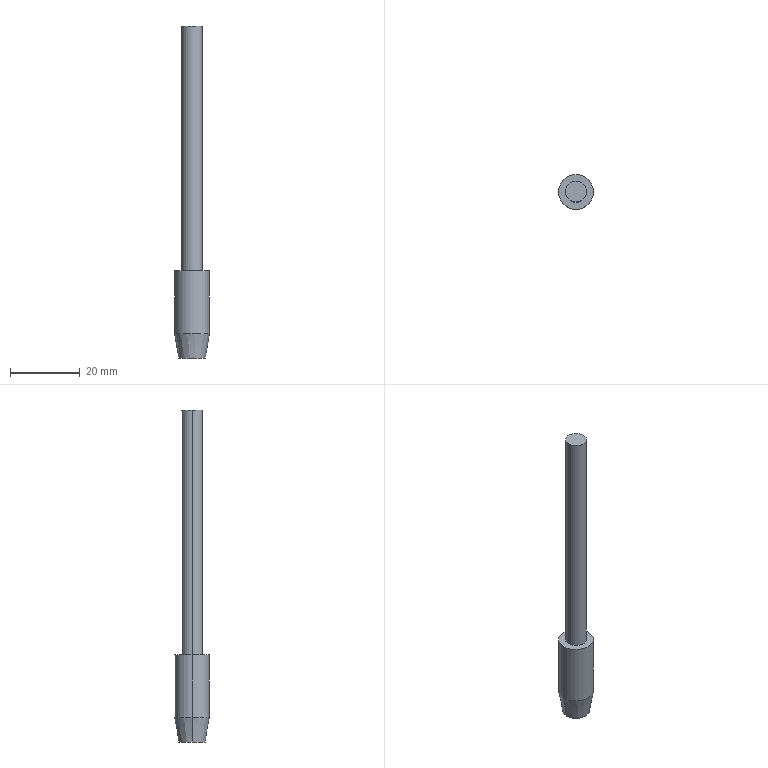Part | STEP file | Traction holder locating screw QY-1-40 | 1 solid | 9 faces | box 10 x 10 x 95 mm | volume 3821 mm3 | cylinder 4 | plane 3 | cone 2 | commonest cylinder face diameters 6 x2 10 x2
STEP:
#1=CARTESIAN_POINT('',(0.,0.,0.));
#2=DIRECTION('',(0.,0.,1.));
#3=DIRECTION('',(1.,0.,0.));
#4=AXIS2_PLACEMENT_3D('',#1,#2,#3);
#5=CARTESIAN_POINT('',(-3.8,0.,0.));
#6=VERTEX_POINT('',#5);
#7=CARTESIAN_POINT('',(3.8,0.,0.));
#8=VERTEX_POINT('',#7);
#9=CARTESIAN_POINT('',(0.,0.,0.));
#10=DIRECTION('',(0.,0.,-1.));
#11=DIRECTION('',(-1.,0.,0.));
#12=AXIS2_PLACEMENT_3D('',#9,#10,#11);
#13=CIRCLE('',#12,3.8);
#14=CARTESIAN_POINT('',(0.,0.,7.));
#15=DIRECTION('',(0.,0.,1.));
#16=DIRECTION('',(1.,0.,0.));
#17=AXIS2_PLACEMENT_3D('',#14,#15,#16);
#18=CONICAL_SURFACE('',#17,5.,0.1698);
#19=CARTESIAN_POINT('',(3.142,-7.));
#20=DIRECTION('',(-1.,0.));
#21=VECTOR('',#20,1.);
#22=LINE('',#19,#21);
#23=(GEOMETRIC_REPRESENTATION_CONTEXT(2)PARAMETRIC_REPRESENTATION_CONTEXT()REPRESENTATION_CONTEXT('',''));
#24=DEFINITIONAL_REPRESENTATION('',(#22),#23);
#25=PCURVE('',#18,#24);
#26=CARTESIAN_POINT('',(0.,0.,0.));
#27=DIRECTION('',(0.,0.,1.));
#28=DIRECTION('',(1.,0.,0.));
#29=AXIS2_PLACEMENT_3D('',#26,#27,#28);
#30=PLANE('',#29);
#31=CARTESIAN_POINT('',(-3.8,0.));
#32=CARTESIAN_POINT('',(-3.8,6.582));
#33=CARTESIAN_POINT('',(1.9,3.291));
#34=CARTESIAN_POINT('',(7.6,0.));
#35=CARTESIAN_POINT('',(1.9,-3.291));
#36=CARTESIAN_POINT('',(-3.8,-6.582));
#37=CARTESIAN_POINT('',(-3.8,0.));
#38=(BOUNDED_CURVE()B_SPLINE_CURVE(2,(#31,#32,#33,#34,#35,#36,#37),.UNSPECIFIED.,.T.,.F.)B_SPLINE_CURVE_WITH_KNOTS((1,2,2,2,2,1),(-2.094,0.,2.094,4.189,6.283,8.378),.UNSPECIFIED.)CURVE()GEOMETRIC_REPRESENTATION_ITEM()RATIONAL_B_SPLINE_CURVE((1.,0.5,1.,0.5,1.,0.5,1.))REPRESENTATION_ITEM(''));
#39=(GEOMETRIC_REPRESENTATION_CONTEXT(2)PARAMETRIC_REPRESENTATION_CONTEXT()REPRESENTATION_CONTEXT('',''));
#40=DEFINITIONAL_REPRESENTATION('',(#38),#39);
#41=PCURVE('',#30,#40);
#42=SURFACE_CURVE('',#13,(#25,#41),.PCURVE_S1.);
#43=EDGE_CURVE('',#6,#8,#42,.T.);
#44=ORIENTED_EDGE('',*,*,#43,.F.);
#45=CARTESIAN_POINT('',(-5.,0.,7.));
#46=VERTEX_POINT('',#45);
#47=CARTESIAN_POINT('',(-5.,0.,7.));
#48=DIRECTION('',(-0.169,0.,0.9856));
#49=VECTOR('',#48,1.);
#50=LINE('',#47,#49);
#51=CARTESIAN_POINT('',(3.142,0.));
#52=DIRECTION('',(0.,1.));
#53=VECTOR('',#52,1.);
#54=LINE('',#51,#53);
#55=(GEOMETRIC_REPRESENTATION_CONTEXT(2)PARAMETRIC_REPRESENTATION_CONTEXT()REPRESENTATION_CONTEXT('',''));
#56=DEFINITIONAL_REPRESENTATION('',(#54),#55);
#57=PCURVE('',#18,#56);
#58=CARTESIAN_POINT('',(0.,0.,7.));
#59=DIRECTION('',(0.,0.,1.));
#60=DIRECTION('',(1.,0.,0.));
#61=AXIS2_PLACEMENT_3D('',#58,#59,#60);
#62=CONICAL_SURFACE('',#61,5.,0.1698);
#63=CARTESIAN_POINT('',(3.142,0.));
#64=DIRECTION('',(0.,1.));
#65=VECTOR('',#64,1.);
#66=LINE('',#63,#65);
#67=(GEOMETRIC_REPRESENTATION_CONTEXT(2)PARAMETRIC_REPRESENTATION_CONTEXT()REPRESENTATION_CONTEXT('',''));
#68=DEFINITIONAL_REPRESENTATION('',(#66),#67);
#69=PCURVE('',#62,#68);
#70=SURFACE_CURVE('',#50,(#57,#69),.PCURVE_S1.);
#71=EDGE_CURVE('',#6,#46,#70,.T.);
#72=ORIENTED_EDGE('',*,*,#71,.T.);
#73=CARTESIAN_POINT('',(5.,0.,7.));
#74=VERTEX_POINT('',#73);
#75=CARTESIAN_POINT('',(0.,0.,7.));
#76=DIRECTION('',(0.,0.,-1.));
#77=DIRECTION('',(-1.,0.,0.));
#78=AXIS2_PLACEMENT_3D('',#75,#76,#77);
#79=CIRCLE('',#78,5.);
#80=CARTESIAN_POINT('',(3.142,0.));
#81=DIRECTION('',(-1.,0.));
#82=VECTOR('',#81,1.);
#83=LINE('',#80,#82);
#84=(GEOMETRIC_REPRESENTATION_CONTEXT(2)PARAMETRIC_REPRESENTATION_CONTEXT()REPRESENTATION_CONTEXT('',''));
#85=DEFINITIONAL_REPRESENTATION('',(#83),#84);
#86=PCURVE('',#18,#85);
#87=CARTESIAN_POINT('',(0.,0.,25.));
#88=DIRECTION('',(0.,0.,-1.));
#89=DIRECTION('',(-1.,0.,0.));
#90=AXIS2_PLACEMENT_3D('',#87,#88,#89);
#91=CYLINDRICAL_SURFACE('',#90,5.);
#92=CARTESIAN_POINT('',(0.,18.));
#93=DIRECTION('',(1.,0.));
#94=VECTOR('',#93,1.);
#95=LINE('',#92,#94);
#96=(GEOMETRIC_REPRESENTATION_CONTEXT(2)PARAMETRIC_REPRESENTATION_CONTEXT()REPRESENTATION_CONTEXT('',''));
#97=DEFINITIONAL_REPRESENTATION('',(#95),#96);
#98=PCURVE('',#91,#97);
#99=SURFACE_CURVE('',#79,(#86,#98),.PCURVE_S1.);
#100=EDGE_CURVE('',#46,#74,#99,.T.);
#101=ORIENTED_EDGE('',*,*,#100,.T.);
#102=CARTESIAN_POINT('',(5.,0.,7.));
#103=DIRECTION('',(0.169,0.,0.9856));
#104=VECTOR('',#103,1.);
#105=LINE('',#102,#104);
#106=CARTESIAN_POINT('',(0.,0.));
#107=DIRECTION('',(0.,1.));
#108=VECTOR('',#107,1.);
#109=LINE('',#106,#108);
#110=(GEOMETRIC_REPRESENTATION_CONTEXT(2)PARAMETRIC_REPRESENTATION_CONTEXT()REPRESENTATION_CONTEXT('',''));
#111=DEFINITIONAL_REPRESENTATION('',(#109),#110);
#112=PCURVE('',#18,#111);
#113=CARTESIAN_POINT('',(6.283,0.));
#114=DIRECTION('',(0.,1.));
#115=VECTOR('',#114,1.);
#116=LINE('',#113,#115);
#117=(GEOMETRIC_REPRESENTATION_CONTEXT(2)PARAMETRIC_REPRESENTATION_CONTEXT()REPRESENTATION_CONTEXT('',''));
#118=DEFINITIONAL_REPRESENTATION('',(#116),#117);
#119=PCURVE('',#62,#118);
#120=SURFACE_CURVE('',#105,(#112,#119),.PCURVE_S1.);
#121=EDGE_CURVE('',#8,#74,#120,.T.);
#122=ORIENTED_EDGE('',*,*,#121,.F.);
#123=EDGE_LOOP('',(#44,#72,#101,#122));
#124=FACE_BOUND('',#123,.T.);
#125=ADVANCED_FACE('',(#124),#18,.T.);
#126=CARTESIAN_POINT('',(3.,0.,95.));
#127=VERTEX_POINT('',#126);
#128=CARTESIAN_POINT('',(-3.,0.,95.));
#129=VERTEX_POINT('',#128);
#130=CARTESIAN_POINT('',(0.,0.,95.));
#131=DIRECTION('',(0.,0.,1.));
#132=DIRECTION('',(1.,0.,0.));
#133=AXIS2_PLACEMENT_3D('',#130,#131,#132);
#134=CIRCLE('',#133,3.);
#135=CARTESIAN_POINT('',(0.,0.,95.));
#136=DIRECTION('',(0.,0.,-1.));
#137=DIRECTION('',(-1.,0.,0.));
#138=AXIS2_PLACEMENT_3D('',#135,#136,#137);
#139=CYLINDRICAL_SURFACE('',#138,3.);
#140=CARTESIAN_POINT('',(3.142,0.));
#141=DIRECTION('',(-1.,0.));
#142=VECTOR('',#141,1.);
#143=LINE('',#140,#142);
#144=(GEOMETRIC_REPRESENTATION_CONTEXT(2)PARAMETRIC_REPRESENTATION_CONTEXT()REPRESENTATION_CONTEXT('',''));
#145=DEFINITIONAL_REPRESENTATION('',(#143),#144);
#146=PCURVE('',#139,#145);
#147=CARTESIAN_POINT('',(0.,0.,95.));
#148=DIRECTION('',(0.,0.,1.));
#149=DIRECTION('',(1.,0.,0.));
#150=AXIS2_PLACEMENT_3D('',#147,#148,#149);
#151=PLANE('',#150);
#152=CARTESIAN_POINT('',(0.,0.));
#153=DIRECTION('',(1.,0.));
#154=AXIS2_PLACEMENT_2D('',#152,#153);
#155=CIRCLE('',#154,3.);
#156=(GEOMETRIC_REPRESENTATION_CONTEXT(2)PARAMETRIC_REPRESENTATION_CONTEXT()REPRESENTATION_CONTEXT('',''));
#157=DEFINITIONAL_REPRESENTATION('',(#155),#156);
#158=PCURVE('',#151,#157);
#159=SURFACE_CURVE('',#134,(#146,#158),.PCURVE_S1.);
#160=EDGE_CURVE('',#127,#129,#159,.T.);
#161=ORIENTED_EDGE('',*,*,#160,.F.);
#162=CARTESIAN_POINT('',(3.,0.,25.));
#163=VERTEX_POINT('',#162);
#164=CARTESIAN_POINT('',(3.,0.,95.));
#165=DIRECTION('',(0.,0.,-1.));
#166=VECTOR('',#165,1.);
#167=LINE('',#164,#166);
#168=CARTESIAN_POINT('',(3.142,0.));
#169=DIRECTION('',(0.,1.));
#170=VECTOR('',#169,1.);
#171=LINE('',#168,#170);
#172=(GEOMETRIC_REPRESENTATION_CONTEXT(2)PARAMETRIC_REPRESENTATION_CONTEXT()REPRESENTATION_CONTEXT('',''));
#173=DEFINITIONAL_REPRESENTATION('',(#171),#172);
#174=PCURVE('',#139,#173);
#175=CARTESIAN_POINT('',(0.,0.,95.));
#176=DIRECTION('',(0.,0.,-1.));
#177=DIRECTION('',(-1.,0.,0.));
#178=AXIS2_PLACEMENT_3D('',#175,#176,#177);
#179=CYLINDRICAL_SURFACE('',#178,3.);
#180=CARTESIAN_POINT('',(3.142,0.));
#181=DIRECTION('',(0.,1.));
#182=VECTOR('',#181,1.);
#183=LINE('',#180,#182);
#184=(GEOMETRIC_REPRESENTATION_CONTEXT(2)PARAMETRIC_REPRESENTATION_CONTEXT()REPRESENTATION_CONTEXT('',''));
#185=DEFINITIONAL_REPRESENTATION('',(#183),#184);
#186=PCURVE('',#179,#185);
#187=SURFACE_CURVE('',#167,(#174,#186),.PCURVE_S1.);
#188=EDGE_CURVE('',#127,#163,#187,.T.);
#189=ORIENTED_EDGE('',*,*,#188,.T.);
#190=CARTESIAN_POINT('',(-3.,0.,25.));
#191=VERTEX_POINT('',#190);
#192=CARTESIAN_POINT('',(0.,0.,25.));
#193=DIRECTION('',(0.,0.,1.));
#194=DIRECTION('',(1.,0.,0.));
#195=AXIS2_PLACEMENT_3D('',#192,#193,#194);
#196=CIRCLE('',#195,3.);
#197=CARTESIAN_POINT('',(3.142,70.));
#198=DIRECTION('',(-1.,0.));
#199=VECTOR('',#198,1.);
#200=LINE('',#197,#199);
#201=(GEOMETRIC_REPRESENTATION_CONTEXT(2)PARAMETRIC_REPRESENTATION_CONTEXT()REPRESENTATION_CONTEXT('',''));
#202=DEFINITIONAL_REPRESENTATION('',(#200),#201);
#203=PCURVE('',#139,#202);
#204=CARTESIAN_POINT('',(0.,0.,25.));
#205=DIRECTION('',(0.,0.,1.));
#206=DIRECTION('',(1.,0.,0.));
#207=AXIS2_PLACEMENT_3D('',#204,#205,#206);
#208=PLANE('',#207);
#209=CARTESIAN_POINT('',(0.,0.));
#210=DIRECTION('',(1.,0.));
#211=AXIS2_PLACEMENT_2D('',#209,#210);
#212=CIRCLE('',#211,3.);
#213=(GEOMETRIC_REPRESENTATION_CONTEXT(2)PARAMETRIC_REPRESENTATION_CONTEXT()REPRESENTATION_CONTEXT('',''));
#214=DEFINITIONAL_REPRESENTATION('',(#212),#213);
#215=PCURVE('',#208,#214);
#216=SURFACE_CURVE('',#196,(#203,#215),.PCURVE_S1.);
#217=EDGE_CURVE('',#163,#191,#216,.T.);
#218=ORIENTED_EDGE('',*,*,#217,.T.);
#219=CARTESIAN_POINT('',(-3.,0.,95.));
#220=DIRECTION('',(0.,0.,-1.));
#221=VECTOR('',#220,1.);
#222=LINE('',#219,#221);
#223=CARTESIAN_POINT('',(0.,0.));
#224=DIRECTION('',(0.,1.));
#225=VECTOR('',#224,1.);
#226=LINE('',#223,#225);
#227=(GEOMETRIC_REPRESENTATION_CONTEXT(2)PARAMETRIC_REPRESENTATION_CONTEXT()REPRESENTATION_CONTEXT('',''));
#228=DEFINITIONAL_REPRESENTATION('',(#226),#227);
#229=PCURVE('',#139,#228);
#230=CARTESIAN_POINT('',(6.283,0.));
#231=DIRECTION('',(0.,1.));
#232=VECTOR('',#231,1.);
#233=LINE('',#230,#232);
#234=(GEOMETRIC_REPRESENTATION_CONTEXT(2)PARAMETRIC_REPRESENTATION_CONTEXT()REPRESENTATION_CONTEXT('',''));
#235=DEFINITIONAL_REPRESENTATION('',(#233),#234);
#236=PCURVE('',#179,#235);
#237=SURFACE_CURVE('',#222,(#229,#236),.PCURVE_S1.);
#238=EDGE_CURVE('',#129,#191,#237,.T.);
#239=ORIENTED_EDGE('',*,*,#238,.F.);
#240=EDGE_LOOP('',(#161,#189,#218,#239));
#241=FACE_BOUND('',#240,.T.);
#242=ADVANCED_FACE('',(#241),#139,.T.);
#243=CARTESIAN_POINT('',(5.,0.,25.));
#244=VERTEX_POINT('',#243);
#245=CARTESIAN_POINT('',(-5.,0.,25.));
#246=VERTEX_POINT('',#245);
#247=CARTESIAN_POINT('',(0.,0.,25.));
#248=DIRECTION('',(0.,0.,1.));
#249=DIRECTION('',(1.,0.,0.));
#250=AXIS2_PLACEMENT_3D('',#247,#248,#249);
#251=CIRCLE('',#250,5.);
#252=CARTESIAN_POINT('',(3.142,0.));
#253=DIRECTION('',(-1.,0.));
#254=VECTOR('',#253,1.);
#255=LINE('',#252,#254);
#256=(GEOMETRIC_REPRESENTATION_CONTEXT(2)PARAMETRIC_REPRESENTATION_CONTEXT()REPRESENTATION_CONTEXT('',''));
#257=DEFINITIONAL_REPRESENTATION('',(#255),#256);
#258=PCURVE('',#91,#257);
#259=CARTESIAN_POINT('',(0.,0.));
#260=DIRECTION('',(1.,0.));
#261=AXIS2_PLACEMENT_2D('',#259,#260);
#262=CIRCLE('',#261,5.);
#263=(GEOMETRIC_REPRESENTATION_CONTEXT(2)PARAMETRIC_REPRESENTATION_CONTEXT()REPRESENTATION_CONTEXT('',''));
#264=DEFINITIONAL_REPRESENTATION('',(#262),#263);
#265=PCURVE('',#208,#264);
#266=SURFACE_CURVE('',#251,(#258,#265),.PCURVE_S1.);
#267=EDGE_CURVE('',#244,#246,#266,.T.);
#268=ORIENTED_EDGE('',*,*,#267,.F.);
#269=CARTESIAN_POINT('',(5.,0.,25.));
#270=DIRECTION('',(0.,0.,-1.));
#271=VECTOR('',#270,1.);
#272=LINE('',#269,#271);
#273=CARTESIAN_POINT('',(3.142,0.));
#274=DIRECTION('',(0.,1.));
#275=VECTOR('',#274,1.);
#276=LINE('',#273,#275);
#277=(GEOMETRIC_REPRESENTATION_CONTEXT(2)PARAMETRIC_REPRESENTATION_CONTEXT()REPRESENTATION_CONTEXT('',''));
#278=DEFINITIONAL_REPRESENTATION('',(#276),#277);
#279=PCURVE('',#91,#278);
#280=CARTESIAN_POINT('',(0.,0.,25.));
#281=DIRECTION('',(0.,0.,-1.));
#282=DIRECTION('',(-1.,0.,0.));
#283=AXIS2_PLACEMENT_3D('',#280,#281,#282);
#284=CYLINDRICAL_SURFACE('',#283,5.);
#285=CARTESIAN_POINT('',(3.142,0.));
#286=DIRECTION('',(0.,1.));
#287=VECTOR('',#286,1.);
#288=LINE('',#285,#287);
#289=(GEOMETRIC_REPRESENTATION_CONTEXT(2)PARAMETRIC_REPRESENTATION_CONTEXT()REPRESENTATION_CONTEXT('',''));
#290=DEFINITIONAL_REPRESENTATION('',(#288),#289);
#291=PCURVE('',#284,#290);
#292=SURFACE_CURVE('',#272,(#279,#291),.PCURVE_S1.);
#293=EDGE_CURVE('',#244,#74,#292,.T.);
#294=ORIENTED_EDGE('',*,*,#293,.T.);
#295=ORIENTED_EDGE('',*,*,#100,.F.);
#296=CARTESIAN_POINT('',(-5.,0.,25.));
#297=DIRECTION('',(0.,0.,-1.));
#298=VECTOR('',#297,1.);
#299=LINE('',#296,#298);
#300=CARTESIAN_POINT('',(0.,0.));
#301=DIRECTION('',(0.,1.));
#302=VECTOR('',#301,1.);
#303=LINE('',#300,#302);
#304=(GEOMETRIC_REPRESENTATION_CONTEXT(2)PARAMETRIC_REPRESENTATION_CONTEXT()REPRESENTATION_CONTEXT('',''));
#305=DEFINITIONAL_REPRESENTATION('',(#303),#304);
#306=PCURVE('',#91,#305);
#307=CARTESIAN_POINT('',(6.283,0.));
#308=DIRECTION('',(0.,1.));
#309=VECTOR('',#308,1.);
#310=LINE('',#307,#309);
#311=(GEOMETRIC_REPRESENTATION_CONTEXT(2)PARAMETRIC_REPRESENTATION_CONTEXT()REPRESENTATION_CONTEXT('',''));
#312=DEFINITIONAL_REPRESENTATION('',(#310),#311);
#313=PCURVE('',#284,#312);
#314=SURFACE_CURVE('',#299,(#306,#313),.PCURVE_S1.);
#315=EDGE_CURVE('',#246,#46,#314,.T.);
#316=ORIENTED_EDGE('',*,*,#315,.F.);
#317=EDGE_LOOP('',(#268,#294,#295,#316));
#318=FACE_BOUND('',#317,.T.);
#319=ADVANCED_FACE('',(#318),#91,.T.);
#320=ORIENTED_EDGE('',*,*,#293,.F.);
#321=CARTESIAN_POINT('',(0.,0.,25.));
#322=DIRECTION('',(0.,0.,1.));
#323=DIRECTION('',(1.,0.,0.));
#324=AXIS2_PLACEMENT_3D('',#321,#322,#323);
#325=CIRCLE('',#324,5.);
#326=CARTESIAN_POINT('',(9.425,0.));
#327=DIRECTION('',(-1.,0.));
#328=VECTOR('',#327,1.);
#329=LINE('',#326,#328);
#330=(GEOMETRIC_REPRESENTATION_CONTEXT(2)PARAMETRIC_REPRESENTATION_CONTEXT()REPRESENTATION_CONTEXT('',''));
#331=DEFINITIONAL_REPRESENTATION('',(#329),#330);
#332=PCURVE('',#284,#331);
#333=CARTESIAN_POINT('',(0.,0.));
#334=DIRECTION('',(1.,0.));
#335=AXIS2_PLACEMENT_2D('',#333,#334);
#336=CIRCLE('',#335,5.);
#337=(GEOMETRIC_REPRESENTATION_CONTEXT(2)PARAMETRIC_REPRESENTATION_CONTEXT()REPRESENTATION_CONTEXT('',''));
#338=DEFINITIONAL_REPRESENTATION('',(#336),#337);
#339=PCURVE('',#208,#338);
#340=SURFACE_CURVE('',#325,(#332,#339),.PCURVE_S1.);
#341=EDGE_CURVE('',#246,#244,#340,.T.);
#342=ORIENTED_EDGE('',*,*,#341,.F.);
#343=ORIENTED_EDGE('',*,*,#315,.T.);
#344=CARTESIAN_POINT('',(0.,0.,7.));
#345=DIRECTION('',(0.,0.,-1.));
#346=DIRECTION('',(-1.,0.,0.));
#347=AXIS2_PLACEMENT_3D('',#344,#345,#346);
#348=CIRCLE('',#347,5.);
#349=CARTESIAN_POINT('',(0.,18.));
#350=DIRECTION('',(1.,0.));
#351=VECTOR('',#350,1.);
#352=LINE('',#349,#351);
#353=(GEOMETRIC_REPRESENTATION_CONTEXT(2)PARAMETRIC_REPRESENTATION_CONTEXT()REPRESENTATION_CONTEXT('',''));
#354=DEFINITIONAL_REPRESENTATION('',(#352),#353);
#355=PCURVE('',#284,#354);
#356=CARTESIAN_POINT('',(9.425,0.));
#357=DIRECTION('',(-1.,0.));
#358=VECTOR('',#357,1.);
#359=LINE('',#356,#358);
#360=(GEOMETRIC_REPRESENTATION_CONTEXT(2)PARAMETRIC_REPRESENTATION_CONTEXT()REPRESENTATION_CONTEXT('',''));
#361=DEFINITIONAL_REPRESENTATION('',(#359),#360);
#362=PCURVE('',#62,#361);
#363=SURFACE_CURVE('',#348,(#355,#362),.PCURVE_S1.);
#364=EDGE_CURVE('',#74,#46,#363,.T.);
#365=ORIENTED_EDGE('',*,*,#364,.F.);
#366=EDGE_LOOP('',(#320,#342,#343,#365));
#367=FACE_BOUND('',#366,.T.);
#368=ADVANCED_FACE('',(#367),#284,.T.);
#369=CARTESIAN_POINT('',(0.,0.,25.));
#370=DIRECTION('',(0.,0.,1.));
#371=DIRECTION('',(1.,0.,0.));
#372=AXIS2_PLACEMENT_3D('',#369,#370,#371);
#373=CIRCLE('',#372,3.);
#374=CARTESIAN_POINT('',(0.,0.));
#375=DIRECTION('',(1.,0.));
#376=AXIS2_PLACEMENT_2D('',#374,#375);
#377=CIRCLE('',#376,3.);
#378=(GEOMETRIC_REPRESENTATION_CONTEXT(2)PARAMETRIC_REPRESENTATION_CONTEXT()REPRESENTATION_CONTEXT('',''));
#379=DEFINITIONAL_REPRESENTATION('',(#377),#378);
#380=PCURVE('',#208,#379);
#381=CARTESIAN_POINT('',(9.425,70.));
#382=DIRECTION('',(-1.,0.));
#383=VECTOR('',#382,1.);
#384=LINE('',#381,#383);
#385=(GEOMETRIC_REPRESENTATION_CONTEXT(2)PARAMETRIC_REPRESENTATION_CONTEXT()REPRESENTATION_CONTEXT('',''));
#386=DEFINITIONAL_REPRESENTATION('',(#384),#385);
#387=PCURVE('',#179,#386);
#388=SURFACE_CURVE('',#373,(#380,#387),.PCURVE_S1.);
#389=EDGE_CURVE('',#191,#163,#388,.T.);
#390=ORIENTED_EDGE('',*,*,#389,.F.);
#391=ORIENTED_EDGE('',*,*,#217,.F.);
#392=EDGE_LOOP('',(#390,#391));
#393=FACE_BOUND('',#392,.T.);
#394=ORIENTED_EDGE('',*,*,#341,.T.);
#395=ORIENTED_EDGE('',*,*,#267,.T.);
#396=EDGE_LOOP('',(#394,#395));
#397=FACE_BOUND('',#396,.T.);
#398=ADVANCED_FACE('',(#393,#397),#208,.T.);
#399=ORIENTED_EDGE('',*,*,#188,.F.);
#400=CARTESIAN_POINT('',(0.,0.,95.));
#401=DIRECTION('',(0.,0.,1.));
#402=DIRECTION('',(1.,0.,0.));
#403=AXIS2_PLACEMENT_3D('',#400,#401,#402);
#404=CIRCLE('',#403,3.);
#405=CARTESIAN_POINT('',(9.425,0.));
#406=DIRECTION('',(-1.,0.));
#407=VECTOR('',#406,1.);
#408=LINE('',#405,#407);
#409=(GEOMETRIC_REPRESENTATION_CONTEXT(2)PARAMETRIC_REPRESENTATION_CONTEXT()REPRESENTATION_CONTEXT('',''));
#410=DEFINITIONAL_REPRESENTATION('',(#408),#409);
#411=PCURVE('',#179,#410);
#412=CARTESIAN_POINT('',(0.,0.));
#413=DIRECTION('',(1.,0.));
#414=AXIS2_PLACEMENT_2D('',#412,#413);
#415=CIRCLE('',#414,3.);
#416=(GEOMETRIC_REPRESENTATION_CONTEXT(2)PARAMETRIC_REPRESENTATION_CONTEXT()REPRESENTATION_CONTEXT('',''));
#417=DEFINITIONAL_REPRESENTATION('',(#415),#416);
#418=PCURVE('',#151,#417);
#419=SURFACE_CURVE('',#404,(#411,#418),.PCURVE_S1.);
#420=EDGE_CURVE('',#129,#127,#419,.T.);
#421=ORIENTED_EDGE('',*,*,#420,.F.);
#422=ORIENTED_EDGE('',*,*,#238,.T.);
#423=ORIENTED_EDGE('',*,*,#389,.T.);
#424=EDGE_LOOP('',(#399,#421,#422,#423));
#425=FACE_BOUND('',#424,.T.);
#426=ADVANCED_FACE('',(#425),#179,.T.);
#427=ORIENTED_EDGE('',*,*,#420,.T.);
#428=ORIENTED_EDGE('',*,*,#160,.T.);
#429=EDGE_LOOP('',(#427,#428));
#430=FACE_BOUND('',#429,.T.);
#431=ADVANCED_FACE('',(#430),#151,.T.);
#432=ORIENTED_EDGE('',*,*,#71,.F.);
#433=CARTESIAN_POINT('',(0.,0.,0.));
#434=DIRECTION('',(0.,0.,-1.));
#435=DIRECTION('',(-1.,0.,0.));
#436=AXIS2_PLACEMENT_3D('',#433,#434,#435);
#437=CIRCLE('',#436,3.8);
#438=CARTESIAN_POINT('',(9.425,-7.));
#439=DIRECTION('',(-1.,0.));
#440=VECTOR('',#439,1.);
#441=LINE('',#438,#440);
#442=(GEOMETRIC_REPRESENTATION_CONTEXT(2)PARAMETRIC_REPRESENTATION_CONTEXT()REPRESENTATION_CONTEXT('',''));
#443=DEFINITIONAL_REPRESENTATION('',(#441),#442);
#444=PCURVE('',#62,#443);
#445=CARTESIAN_POINT('',(-3.8,0.));
#446=CARTESIAN_POINT('',(-3.8,6.582));
#447=CARTESIAN_POINT('',(1.9,3.291));
#448=CARTESIAN_POINT('',(7.6,0.));
#449=CARTESIAN_POINT('',(1.9,-3.291));
#450=CARTESIAN_POINT('',(-3.8,-6.582));
#451=CARTESIAN_POINT('',(-3.8,0.));
#452=(BOUNDED_CURVE()B_SPLINE_CURVE(2,(#445,#446,#447,#448,#449,#450,#451),.UNSPECIFIED.,.T.,.F.)B_SPLINE_CURVE_WITH_KNOTS((1,2,2,2,2,1),(-2.094,0.,2.094,4.189,6.283,8.378),.UNSPECIFIED.)CURVE()GEOMETRIC_REPRESENTATION_ITEM()RATIONAL_B_SPLINE_CURVE((1.,0.5,1.,0.5,1.,0.5,1.))REPRESENTATION_ITEM(''));
#453=(GEOMETRIC_REPRESENTATION_CONTEXT(2)PARAMETRIC_REPRESENTATION_CONTEXT()REPRESENTATION_CONTEXT('',''));
#454=DEFINITIONAL_REPRESENTATION('',(#452),#453);
#455=PCURVE('',#30,#454);
#456=SURFACE_CURVE('',#437,(#444,#455),.PCURVE_S1.);
#457=EDGE_CURVE('',#8,#6,#456,.T.);
#458=ORIENTED_EDGE('',*,*,#457,.F.);
#459=ORIENTED_EDGE('',*,*,#121,.T.);
#460=ORIENTED_EDGE('',*,*,#364,.T.);
#461=EDGE_LOOP('',(#432,#458,#459,#460));
#462=FACE_BOUND('',#461,.T.);
#463=ADVANCED_FACE('',(#462),#62,.T.);
#464=ORIENTED_EDGE('',*,*,#457,.T.);
#465=ORIENTED_EDGE('',*,*,#43,.T.);
#466=EDGE_LOOP('',(#464,#465));
#467=FACE_BOUND('',#466,.T.);
#468=ADVANCED_FACE('',(#467),#30,.F.);
#469=CLOSED_SHELL('',(#125,#242,#319,#368,#398,#426,#431,#463,#468));
#470=MANIFOLD_SOLID_BREP('',#469);
#471=(LENGTH_UNIT()NAMED_UNIT(*)SI_UNIT(.MILLI.,.METRE.));
#472=UNCERTAINTY_MEASURE_WITH_UNIT(LENGTH_MEASURE(0.0000001),#471,'','');
#473=(NAMED_UNIT(*)PLANE_ANGLE_UNIT()SI_UNIT($,.RADIAN.));
#474=(NAMED_UNIT(*)SI_UNIT($,.STERADIAN.)SOLID_ANGLE_UNIT());
#475=(GEOMETRIC_REPRESENTATION_CONTEXT(3)GLOBAL_UNCERTAINTY_ASSIGNED_CONTEXT((#472))GLOBAL_UNIT_ASSIGNED_CONTEXT((#471,#473,#474))REPRESENTATION_CONTEXT('',''));
#476=ADVANCED_BREP_SHAPE_REPRESENTATION('',(#4,#470),#475);